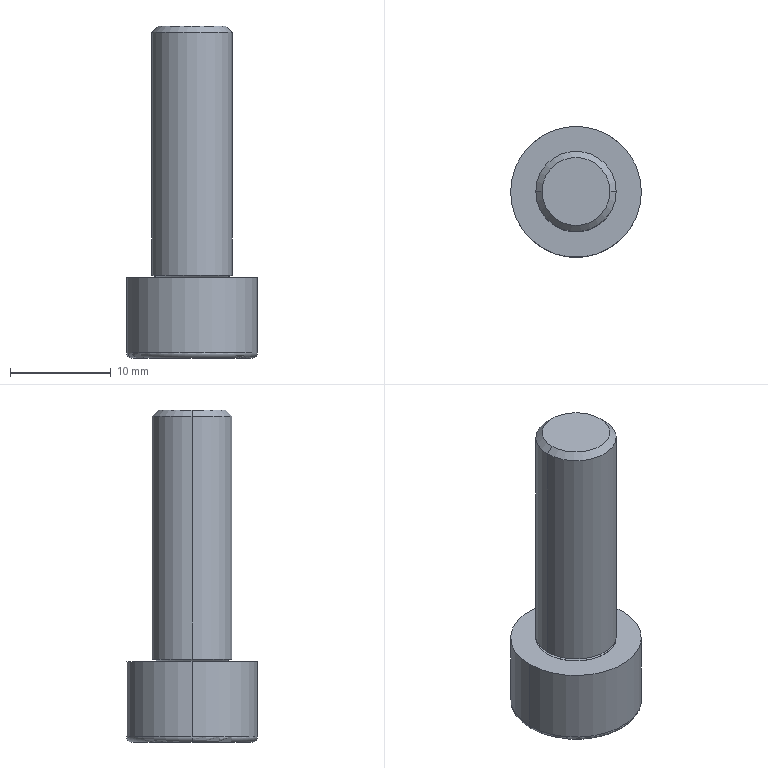Part | SolidWorks | features Attribute 1, Cut 1, Revolution 1 | 1 solid | 27 faces | box 13 x 13 x 33 mm | volume 2217 mm3 | plane 11 | torus 6 | cylinder 6 | cone 4 | commonest cylinder face diameters 8 x4 13 x2
STEP:
#1=CARTESIAN_POINT('',(-3.488,0.,0.01));
#2=VERTEX_POINT('',#1);
#3=CARTESIAN_POINT('',(-3.468,0.,0.03));
#4=VERTEX_POINT('',#3);
#5=CARTESIAN_POINT('',(-3.488,0.,0.03));
#6=DIRECTION('',(0.,-1.,0.));
#7=DIRECTION('',(0.,0.,-1.));
#8=AXIS2_PLACEMENT_3D('',#5,#6,#7);
#9=CIRCLE('',#8,0.02);
#10=EDGE_CURVE('',#2,#4,#9,.T.);
#11=ORIENTED_EDGE('',*,*,#10,.T.);
#12=CARTESIAN_POINT('',(3.468,0.,0.03));
#13=VERTEX_POINT('',#12);
#14=CARTESIAN_POINT('',(0.,0.,0.03));
#15=DIRECTION('',(0.,0.,-1.));
#16=DIRECTION('',(-1.,0.,0.));
#17=AXIS2_PLACEMENT_3D('',#14,#15,#16);
#18=CIRCLE('',#17,3.468);
#19=EDGE_CURVE('',#4,#13,#18,.T.);
#20=ORIENTED_EDGE('',*,*,#19,.T.);
#21=CARTESIAN_POINT('',(3.488,0.,0.01));
#22=VERTEX_POINT('',#21);
#23=CARTESIAN_POINT('',(3.488,0.,0.03));
#24=DIRECTION('',(0.,1.,0.));
#25=DIRECTION('',(-1.,0.,0.));
#26=AXIS2_PLACEMENT_3D('',#23,#24,#25);
#27=CIRCLE('',#26,0.02);
#28=EDGE_CURVE('',#22,#13,#27,.T.);
#29=ORIENTED_EDGE('',*,*,#28,.F.);
#30=CARTESIAN_POINT('',(0.,0.,0.01));
#31=DIRECTION('',(0.,0.,-1.));
#32=DIRECTION('',(-1.,0.,0.));
#33=AXIS2_PLACEMENT_3D('',#30,#31,#32);
#34=CIRCLE('',#33,3.488);
#35=EDGE_CURVE('',#2,#22,#34,.T.);
#36=ORIENTED_EDGE('',*,*,#35,.F.);
#37=EDGE_LOOP('',(#11,#20,#29,#36));
#38=FACE_OUTER_BOUND('',#37,.T.);
#39=CARTESIAN_POINT('',(0.,0.,0.03));
#40=DIRECTION('',(0.,0.,-1.));
#41=DIRECTION('',(-1.,0.,0.));
#42=AXIS2_PLACEMENT_3D('',#39,#40,#41);
#43=TOROIDAL_SURFACE('',#42,3.488,0.02);
#44=ADVANCED_FACE('',(#38),#43,.F.);
#45=ORIENTED_EDGE('',*,*,#28,.T.);
#46=CARTESIAN_POINT('',(0.,0.,0.03));
#47=DIRECTION('',(0.,0.,-1.));
#48=DIRECTION('',(-1.,0.,0.));
#49=AXIS2_PLACEMENT_3D('',#46,#47,#48);
#50=CIRCLE('',#49,3.468);
#51=EDGE_CURVE('',#13,#4,#50,.T.);
#52=ORIENTED_EDGE('',*,*,#51,.T.);
#53=ORIENTED_EDGE('',*,*,#10,.F.);
#54=CARTESIAN_POINT('',(0.,0.,0.01));
#55=DIRECTION('',(0.,0.,-1.));
#56=DIRECTION('',(-1.,0.,0.));
#57=AXIS2_PLACEMENT_3D('',#54,#55,#56);
#58=CIRCLE('',#57,3.488);
#59=EDGE_CURVE('',#22,#2,#58,.T.);
#60=ORIENTED_EDGE('',*,*,#59,.F.);
#61=EDGE_LOOP('',(#45,#52,#53,#60));
#62=FACE_OUTER_BOUND('',#61,.T.);
#63=CARTESIAN_POINT('',(0.,0.,0.03));
#64=DIRECTION('',(0.,0.,-1.));
#65=DIRECTION('',(-1.,0.,0.));
#66=AXIS2_PLACEMENT_3D('',#63,#64,#65);
#67=TOROIDAL_SURFACE('',#66,3.488,0.02);
#68=ADVANCED_FACE('',(#62),#67,.F.);
#69=CARTESIAN_POINT('',(-3.375,0.,25.));
#70=VERTEX_POINT('',#69);
#71=CARTESIAN_POINT('',(3.375,0.,25.));
#72=VERTEX_POINT('',#71);
#73=CARTESIAN_POINT('',(0.,0.,25.));
#74=DIRECTION('',(0.,0.,-1.));
#75=DIRECTION('',(-1.,0.,0.));
#76=AXIS2_PLACEMENT_3D('',#73,#74,#75);
#77=CIRCLE('',#76,3.375);
#78=EDGE_CURVE('',#70,#72,#77,.T.);
#79=ORIENTED_EDGE('',*,*,#78,.T.);
#80=CARTESIAN_POINT('',(4.,0.,24.375));
#81=VERTEX_POINT('',#80);
#82=CARTESIAN_POINT('',(3.375,0.,25.));
#83=DIRECTION('',(0.7071,0.,-0.7071));
#84=VECTOR('',#83,1000.);
#85=LINE('',#82,#84);
#86=EDGE_CURVE('',#72,#81,#85,.T.);
#87=ORIENTED_EDGE('',*,*,#86,.T.);
#88=CARTESIAN_POINT('',(-4.,0.,24.375));
#89=VERTEX_POINT('',#88);
#90=CARTESIAN_POINT('',(0.,0.,24.375));
#91=DIRECTION('',(0.,0.,-1.));
#92=DIRECTION('',(-1.,0.,0.));
#93=AXIS2_PLACEMENT_3D('',#90,#91,#92);
#94=CIRCLE('',#93,4.);
#95=EDGE_CURVE('',#89,#81,#94,.T.);
#96=ORIENTED_EDGE('',*,*,#95,.F.);
#97=CARTESIAN_POINT('',(-3.375,0.,25.));
#98=DIRECTION('',(-0.7071,0.,-0.7071));
#99=VECTOR('',#98,1000.);
#100=LINE('',#97,#99);
#101=EDGE_CURVE('',#70,#89,#100,.T.);
#102=ORIENTED_EDGE('',*,*,#101,.F.);
#103=EDGE_LOOP('',(#79,#87,#96,#102));
#104=FACE_OUTER_BOUND('',#103,.T.);
#105=CARTESIAN_POINT('',(0.,0.,25.));
#106=DIRECTION('',(0.,0.,-1.));
#107=DIRECTION('',(-1.,0.,0.));
#108=AXIS2_PLACEMENT_3D('',#105,#106,#107);
#109=CONICAL_SURFACE('',#108,3.375,0.7854);
#110=ADVANCED_FACE('',(#104),#109,.T.);
#111=ORIENTED_EDGE('',*,*,#95,.T.);
#112=CARTESIAN_POINT('',(4.,0.,0.2375));
#113=VERTEX_POINT('',#112);
#114=CARTESIAN_POINT('',(4.,0.,-10.585));
#115=DIRECTION('',(0.,0.,-1.));
#116=VECTOR('',#115,1000.);
#117=LINE('',#114,#116);
#118=EDGE_CURVE('',#81,#113,#117,.T.);
#119=ORIENTED_EDGE('',*,*,#118,.T.);
#120=CARTESIAN_POINT('',(-4.,0.,0.2375));
#121=VERTEX_POINT('',#120);
#122=CARTESIAN_POINT('',(0.,0.,0.2375));
#123=DIRECTION('',(0.,0.,-1.));
#124=DIRECTION('',(-1.,0.,0.));
#125=AXIS2_PLACEMENT_3D('',#122,#123,#124);
#126=CIRCLE('',#125,4.);
#127=EDGE_CURVE('',#121,#113,#126,.T.);
#128=ORIENTED_EDGE('',*,*,#127,.F.);
#129=CARTESIAN_POINT('',(-4.,0.,-10.585));
#130=DIRECTION('',(0.,0.,-1.));
#131=VECTOR('',#130,1000.);
#132=LINE('',#129,#131);
#133=EDGE_CURVE('',#89,#121,#132,.T.);
#134=ORIENTED_EDGE('',*,*,#133,.F.);
#135=EDGE_LOOP('',(#111,#119,#128,#134));
#136=FACE_OUTER_BOUND('',#135,.T.);
#137=CARTESIAN_POINT('',(0.,0.,-10.585));
#138=DIRECTION('',(0.,0.,-1.));
#139=DIRECTION('',(-1.,0.,0.));
#140=AXIS2_PLACEMENT_3D('',#137,#138,#139);
#141=CYLINDRICAL_SURFACE('',#140,4.);
#142=ADVANCED_FACE('',(#136),#141,.T.);
#143=CARTESIAN_POINT('',(-3.482,0.,0.04879));
#144=VERTEX_POINT('',#143);
#145=CARTESIAN_POINT('',(3.482,0.,0.04879));
#146=VERTEX_POINT('',#145);
#147=CARTESIAN_POINT('',(0.,0.,0.04879));
#148=DIRECTION('',(0.,0.,-1.));
#149=DIRECTION('',(-1.,0.,0.));
#150=AXIS2_PLACEMENT_3D('',#147,#148,#149);
#151=CIRCLE('',#150,3.482);
#152=EDGE_CURVE('',#144,#146,#151,.T.);
#153=ORIENTED_EDGE('',*,*,#152,.F.);
#154=CARTESIAN_POINT('',(-4.,0.,0.2375));
#155=DIRECTION('',(-0.9397,0.,0.342));
#156=VECTOR('',#155,1000.);
#157=LINE('',#154,#156);
#158=EDGE_CURVE('',#144,#121,#157,.T.);
#159=ORIENTED_EDGE('',*,*,#158,.T.);
#160=ORIENTED_EDGE('',*,*,#127,.T.);
#161=CARTESIAN_POINT('',(4.,0.,0.2375));
#162=DIRECTION('',(0.9397,0.,0.342));
#163=VECTOR('',#162,1000.);
#164=LINE('',#161,#163);
#165=EDGE_CURVE('',#146,#113,#164,.T.);
#166=ORIENTED_EDGE('',*,*,#165,.F.);
#167=EDGE_LOOP('',(#153,#159,#160,#166));
#168=FACE_OUTER_BOUND('',#167,.T.);
#169=CARTESIAN_POINT('',(0.,0.,0.2375));
#170=DIRECTION('',(0.,0.,1.));
#171=DIRECTION('',(1.,0.,0.));
#172=AXIS2_PLACEMENT_3D('',#169,#170,#171);
#173=CONICAL_SURFACE('',#172,4.,1.222);
#174=ADVANCED_FACE('',(#168),#173,.T.);
#175=ORIENTED_EDGE('',*,*,#51,.F.);
#176=CARTESIAN_POINT('',(3.488,0.,0.03));
#177=DIRECTION('',(0.,1.,0.));
#178=DIRECTION('',(-1.,0.,0.));
#179=AXIS2_PLACEMENT_3D('',#176,#177,#178);
#180=CIRCLE('',#179,0.02);
#181=EDGE_CURVE('',#13,#146,#180,.T.);
#182=ORIENTED_EDGE('',*,*,#181,.T.);
#183=CARTESIAN_POINT('',(0.,0.,0.04879));
#184=DIRECTION('',(0.,0.,-1.));
#185=DIRECTION('',(-1.,0.,0.));
#186=AXIS2_PLACEMENT_3D('',#183,#184,#185);
#187=CIRCLE('',#186,3.482);
#188=EDGE_CURVE('',#146,#144,#187,.T.);
#189=ORIENTED_EDGE('',*,*,#188,.T.);
#190=CARTESIAN_POINT('',(-3.488,0.,0.03));
#191=DIRECTION('',(0.,-1.,0.));
#192=DIRECTION('',(0.,0.,-1.));
#193=AXIS2_PLACEMENT_3D('',#190,#191,#192);
#194=CIRCLE('',#193,0.02);
#195=EDGE_CURVE('',#4,#144,#194,.T.);
#196=ORIENTED_EDGE('',*,*,#195,.F.);
#197=EDGE_LOOP('',(#175,#182,#189,#196));
#198=FACE_OUTER_BOUND('',#197,.T.);
#199=CARTESIAN_POINT('',(0.,0.,0.03));
#200=DIRECTION('',(0.,0.,-1.));
#201=DIRECTION('',(-1.,0.,0.));
#202=AXIS2_PLACEMENT_3D('',#199,#200,#201);
#203=TOROIDAL_SURFACE('',#202,3.488,0.02);
#204=ADVANCED_FACE('',(#198),#203,.F.);
#205=CARTESIAN_POINT('',(-4.,0.,0.01));
#206=VERTEX_POINT('',#205);
#207=CARTESIAN_POINT('',(4.,0.,0.01));
#208=VERTEX_POINT('',#207);
#209=CARTESIAN_POINT('',(0.,0.,0.01));
#210=DIRECTION('',(0.,0.,-1.));
#211=DIRECTION('',(-1.,0.,0.));
#212=AXIS2_PLACEMENT_3D('',#209,#210,#211);
#213=CIRCLE('',#212,4.);
#214=EDGE_CURVE('',#206,#208,#213,.T.);
#215=ORIENTED_EDGE('',*,*,#214,.T.);
#216=CARTESIAN_POINT('',(4.,0.,0.));
#217=VERTEX_POINT('',#216);
#218=CARTESIAN_POINT('',(4.,0.,-10.585));
#219=DIRECTION('',(0.,0.,-1.));
#220=VECTOR('',#219,1000.);
#221=LINE('',#218,#220);
#222=EDGE_CURVE('',#208,#217,#221,.T.);
#223=ORIENTED_EDGE('',*,*,#222,.T.);
#224=CARTESIAN_POINT('',(-4.,0.,0.));
#225=VERTEX_POINT('',#224);
#226=CARTESIAN_POINT('',(0.,0.,0.));
#227=DIRECTION('',(0.,0.,-1.));
#228=DIRECTION('',(-1.,0.,0.));
#229=AXIS2_PLACEMENT_3D('',#226,#227,#228);
#230=CIRCLE('',#229,4.);
#231=EDGE_CURVE('',#225,#217,#230,.T.);
#232=ORIENTED_EDGE('',*,*,#231,.F.);
#233=CARTESIAN_POINT('',(-4.,0.,-10.585));
#234=DIRECTION('',(0.,0.,-1.));
#235=VECTOR('',#234,1000.);
#236=LINE('',#233,#235);
#237=EDGE_CURVE('',#206,#225,#236,.T.);
#238=ORIENTED_EDGE('',*,*,#237,.F.);
#239=EDGE_LOOP('',(#215,#223,#232,#238));
#240=FACE_OUTER_BOUND('',#239,.T.);
#241=CARTESIAN_POINT('',(0.,0.,-10.585));
#242=DIRECTION('',(0.,0.,-1.));
#243=DIRECTION('',(-1.,0.,0.));
#244=AXIS2_PLACEMENT_3D('',#241,#242,#243);
#245=CYLINDRICAL_SURFACE('',#244,4.);
#246=ADVANCED_FACE('',(#240),#245,.T.);
#247=CARTESIAN_POINT('',(-6.5,0.,0.));
#248=VERTEX_POINT('',#247);
#249=CARTESIAN_POINT('',(6.5,0.,0.));
#250=VERTEX_POINT('',#249);
#251=CARTESIAN_POINT('',(0.,0.,0.));
#252=DIRECTION('',(0.,0.,-1.));
#253=DIRECTION('',(-1.,0.,0.));
#254=AXIS2_PLACEMENT_3D('',#251,#252,#253);
#255=CIRCLE('',#254,6.5);
#256=EDGE_CURVE('',#248,#250,#255,.T.);
#257=ORIENTED_EDGE('',*,*,#256,.T.);
#258=CARTESIAN_POINT('',(6.5,0.,-7.5));
#259=VERTEX_POINT('',#258);
#260=CARTESIAN_POINT('',(6.5,0.,-10.585));
#261=DIRECTION('',(0.,0.,-1.));
#262=VECTOR('',#261,1000.);
#263=LINE('',#260,#262);
#264=EDGE_CURVE('',#250,#259,#263,.T.);
#265=ORIENTED_EDGE('',*,*,#264,.T.);
#266=CARTESIAN_POINT('',(-6.5,0.,-7.5));
#267=VERTEX_POINT('',#266);
#268=CARTESIAN_POINT('',(0.,0.,-7.5));
#269=DIRECTION('',(0.,0.,-1.));
#270=DIRECTION('',(-1.,0.,0.));
#271=AXIS2_PLACEMENT_3D('',#268,#269,#270);
#272=CIRCLE('',#271,6.5);
#273=EDGE_CURVE('',#267,#259,#272,.T.);
#274=ORIENTED_EDGE('',*,*,#273,.F.);
#275=CARTESIAN_POINT('',(-6.5,0.,-10.585));
#276=DIRECTION('',(0.,0.,-1.));
#277=VECTOR('',#276,1000.);
#278=LINE('',#275,#277);
#279=EDGE_CURVE('',#248,#267,#278,.T.);
#280=ORIENTED_EDGE('',*,*,#279,.F.);
#281=EDGE_LOOP('',(#257,#265,#274,#280));
#282=FACE_OUTER_BOUND('',#281,.T.);
#283=CARTESIAN_POINT('',(0.,0.,-10.585));
#284=DIRECTION('',(0.,0.,-1.));
#285=DIRECTION('',(-1.,0.,0.));
#286=AXIS2_PLACEMENT_3D('',#283,#284,#285);
#287=CYLINDRICAL_SURFACE('',#286,6.5);
#288=ADVANCED_FACE('',(#282),#287,.T.);
#289=ORIENTED_EDGE('',*,*,#273,.T.);
#290=CARTESIAN_POINT('',(6.,0.,-8.));
#291=VERTEX_POINT('',#290);
#292=CARTESIAN_POINT('',(6.,0.,-7.5));
#293=DIRECTION('',(0.,1.,0.));
#294=DIRECTION('',(-1.,0.,0.));
#295=AXIS2_PLACEMENT_3D('',#292,#293,#294);
#296=CIRCLE('',#295,0.5);
#297=EDGE_CURVE('',#259,#291,#296,.T.);
#298=ORIENTED_EDGE('',*,*,#297,.T.);
#299=CARTESIAN_POINT('',(-6.,0.,-8.));
#300=VERTEX_POINT('',#299);
#301=CARTESIAN_POINT('',(0.,0.,-8.));
#302=DIRECTION('',(0.,0.,-1.));
#303=DIRECTION('',(-1.,0.,0.));
#304=AXIS2_PLACEMENT_3D('',#301,#302,#303);
#305=CIRCLE('',#304,6.);
#306=EDGE_CURVE('',#300,#291,#305,.T.);
#307=ORIENTED_EDGE('',*,*,#306,.F.);
#308=CARTESIAN_POINT('',(-6.,0.,-7.5));
#309=DIRECTION('',(0.,-1.,0.));
#310=DIRECTION('',(0.,0.,-1.));
#311=AXIS2_PLACEMENT_3D('',#308,#309,#310);
#312=CIRCLE('',#311,0.5);
#313=EDGE_CURVE('',#267,#300,#312,.T.);
#314=ORIENTED_EDGE('',*,*,#313,.F.);
#315=EDGE_LOOP('',(#289,#298,#307,#314));
#316=FACE_OUTER_BOUND('',#315,.T.);
#317=CARTESIAN_POINT('',(0.,0.,-7.5));
#318=DIRECTION('',(0.,0.,-1.));
#319=DIRECTION('',(-1.,0.,0.));
#320=AXIS2_PLACEMENT_3D('',#317,#318,#319);
#321=TOROIDAL_SURFACE('',#320,6.,0.5);
#322=ADVANCED_FACE('',(#316),#321,.T.);
#323=ORIENTED_EDGE('',*,*,#297,.F.);
#324=CARTESIAN_POINT('',(0.,0.,-7.5));
#325=DIRECTION('',(0.,0.,-1.));
#326=DIRECTION('',(-1.,0.,0.));
#327=AXIS2_PLACEMENT_3D('',#324,#325,#326);
#328=CIRCLE('',#327,6.5);
#329=EDGE_CURVE('',#259,#267,#328,.T.);
#330=ORIENTED_EDGE('',*,*,#329,.T.);
#331=ORIENTED_EDGE('',*,*,#313,.T.);
#332=CARTESIAN_POINT('',(0.,0.,-8.));
#333=DIRECTION('',(0.,0.,-1.));
#334=DIRECTION('',(-1.,0.,0.));
#335=AXIS2_PLACEMENT_3D('',#332,#333,#334);
#336=CIRCLE('',#335,6.);
#337=EDGE_CURVE('',#291,#300,#336,.T.);
#338=ORIENTED_EDGE('',*,*,#337,.F.);
#339=EDGE_LOOP('',(#323,#330,#331,#338));
#340=FACE_OUTER_BOUND('',#339,.T.);
#341=CARTESIAN_POINT('',(0.,0.,-7.5));
#342=DIRECTION('',(0.,0.,-1.));
#343=DIRECTION('',(-1.,0.,0.));
#344=AXIS2_PLACEMENT_3D('',#341,#342,#343);
#345=TOROIDAL_SURFACE('',#344,6.,0.5);
#346=ADVANCED_FACE('',(#340),#345,.T.);
#347=ORIENTED_EDGE('',*,*,#264,.F.);
#348=CARTESIAN_POINT('',(0.,0.,0.));
#349=DIRECTION('',(0.,0.,-1.));
#350=DIRECTION('',(-1.,0.,0.));
#351=AXIS2_PLACEMENT_3D('',#348,#349,#350);
#352=CIRCLE('',#351,6.5);
#353=EDGE_CURVE('',#250,#248,#352,.T.);
#354=ORIENTED_EDGE('',*,*,#353,.T.);
#355=ORIENTED_EDGE('',*,*,#279,.T.);
#356=ORIENTED_EDGE('',*,*,#329,.F.);
#357=EDGE_LOOP('',(#347,#354,#355,#356));
#358=FACE_OUTER_BOUND('',#357,.T.);
#359=CARTESIAN_POINT('',(0.,0.,-10.585));
#360=DIRECTION('',(0.,0.,-1.));
#361=DIRECTION('',(-1.,0.,0.));
#362=AXIS2_PLACEMENT_3D('',#359,#360,#361);
#363=CYLINDRICAL_SURFACE('',#362,6.5);
#364=ADVANCED_FACE('',(#358),#363,.T.);
#365=ORIENTED_EDGE('',*,*,#256,.F.);
#366=ORIENTED_EDGE('',*,*,#353,.F.);
#367=EDGE_LOOP('',(#365,#366));
#368=FACE_OUTER_BOUND('',#367,.T.);
#369=ORIENTED_EDGE('',*,*,#231,.T.);
#370=CARTESIAN_POINT('',(0.,0.,0.));
#371=DIRECTION('',(0.,0.,-1.));
#372=DIRECTION('',(-1.,0.,0.));
#373=AXIS2_PLACEMENT_3D('',#370,#371,#372);
#374=CIRCLE('',#373,4.);
#375=EDGE_CURVE('',#217,#225,#374,.T.);
#376=ORIENTED_EDGE('',*,*,#375,.T.);
#377=EDGE_LOOP('',(#369,#376));
#378=FACE_BOUND('',#377,.T.);
#379=CARTESIAN_POINT('',(-6.5,0.,0.));
#380=DIRECTION('',(0.,0.,-1.));
#381=DIRECTION('',(-1.,0.,0.));
#382=AXIS2_PLACEMENT_3D('',#379,#380,#381);
#383=PLANE('',#382);
#384=ADVANCED_FACE('',(#368,#378),#383,.F.);
#385=ORIENTED_EDGE('',*,*,#222,.F.);
#386=CARTESIAN_POINT('',(0.,0.,0.01));
#387=DIRECTION('',(0.,0.,-1.));
#388=DIRECTION('',(-1.,0.,0.));
#389=AXIS2_PLACEMENT_3D('',#386,#387,#388);
#390=CIRCLE('',#389,4.);
#391=EDGE_CURVE('',#208,#206,#390,.T.);
#392=ORIENTED_EDGE('',*,*,#391,.T.);
#393=ORIENTED_EDGE('',*,*,#237,.T.);
#394=ORIENTED_EDGE('',*,*,#375,.F.);
#395=EDGE_LOOP('',(#385,#392,#393,#394));
#396=FACE_OUTER_BOUND('',#395,.T.);
#397=CARTESIAN_POINT('',(0.,0.,-10.585));
#398=DIRECTION('',(0.,0.,-1.));
#399=DIRECTION('',(-1.,0.,0.));
#400=AXIS2_PLACEMENT_3D('',#397,#398,#399);
#401=CYLINDRICAL_SURFACE('',#400,4.);
#402=ADVANCED_FACE('',(#396),#401,.T.);
#403=ORIENTED_EDGE('',*,*,#214,.F.);
#404=ORIENTED_EDGE('',*,*,#391,.F.);
#405=EDGE_LOOP('',(#403,#404));
#406=FACE_OUTER_BOUND('',#405,.T.);
#407=ORIENTED_EDGE('',*,*,#35,.T.);
#408=ORIENTED_EDGE('',*,*,#59,.T.);
#409=EDGE_LOOP('',(#407,#408));
#410=FACE_BOUND('',#409,.T.);
#411=CARTESIAN_POINT('',(-4.,0.,0.01));
#412=DIRECTION('',(0.,0.,-1.));
#413=DIRECTION('',(-1.,0.,0.));
#414=AXIS2_PLACEMENT_3D('',#411,#412,#413);
#415=PLANE('',#414);
#416=ADVANCED_FACE('',(#406,#410),#415,.F.);
#417=ORIENTED_EDGE('',*,*,#19,.F.);
#418=ORIENTED_EDGE('',*,*,#195,.T.);
#419=ORIENTED_EDGE('',*,*,#152,.T.);
#420=ORIENTED_EDGE('',*,*,#181,.F.);
#421=EDGE_LOOP('',(#417,#418,#419,#420));
#422=FACE_OUTER_BOUND('',#421,.T.);
#423=CARTESIAN_POINT('',(0.,0.,0.03));
#424=DIRECTION('',(0.,0.,-1.));
#425=DIRECTION('',(-1.,0.,0.));
#426=AXIS2_PLACEMENT_3D('',#423,#424,#425);
#427=TOROIDAL_SURFACE('',#426,3.488,0.02);
#428=ADVANCED_FACE('',(#422),#427,.F.);
#429=ORIENTED_EDGE('',*,*,#158,.F.);
#430=ORIENTED_EDGE('',*,*,#188,.F.);
#431=ORIENTED_EDGE('',*,*,#165,.T.);
#432=CARTESIAN_POINT('',(0.,0.,0.2375));
#433=DIRECTION('',(0.,0.,-1.));
#434=DIRECTION('',(-1.,0.,0.));
#435=AXIS2_PLACEMENT_3D('',#432,#433,#434);
#436=CIRCLE('',#435,4.);
#437=EDGE_CURVE('',#113,#121,#436,.T.);
#438=ORIENTED_EDGE('',*,*,#437,.T.);
#439=EDGE_LOOP('',(#429,#430,#431,#438));
#440=FACE_OUTER_BOUND('',#439,.T.);
#441=CARTESIAN_POINT('',(0.,0.,0.2375));
#442=DIRECTION('',(0.,0.,1.));
#443=DIRECTION('',(1.,0.,0.));
#444=AXIS2_PLACEMENT_3D('',#441,#442,#443);
#445=CONICAL_SURFACE('',#444,4.,1.222);
#446=ADVANCED_FACE('',(#440),#445,.T.);
#447=ORIENTED_EDGE('',*,*,#118,.F.);
#448=CARTESIAN_POINT('',(0.,0.,24.375));
#449=DIRECTION('',(0.,0.,-1.));
#450=DIRECTION('',(-1.,0.,0.));
#451=AXIS2_PLACEMENT_3D('',#448,#449,#450);
#452=CIRCLE('',#451,4.);
#453=EDGE_CURVE('',#81,#89,#452,.T.);
#454=ORIENTED_EDGE('',*,*,#453,.T.);
#455=ORIENTED_EDGE('',*,*,#133,.T.);
#456=ORIENTED_EDGE('',*,*,#437,.F.);
#457=EDGE_LOOP('',(#447,#454,#455,#456));
#458=FACE_OUTER_BOUND('',#457,.T.);
#459=CARTESIAN_POINT('',(0.,0.,-10.585));
#460=DIRECTION('',(0.,0.,-1.));
#461=DIRECTION('',(-1.,0.,0.));
#462=AXIS2_PLACEMENT_3D('',#459,#460,#461);
#463=CYLINDRICAL_SURFACE('',#462,4.);
#464=ADVANCED_FACE('',(#458),#463,.T.);
#465=ORIENTED_EDGE('',*,*,#86,.F.);
#466=CARTESIAN_POINT('',(0.,0.,25.));
#467=DIRECTION('',(0.,0.,-1.));
#468=DIRECTION('',(-1.,0.,0.));
#469=AXIS2_PLACEMENT_3D('',#466,#467,#468);
#470=CIRCLE('',#469,3.375);
#471=EDGE_CURVE('',#72,#70,#470,.T.);
#472=ORIENTED_EDGE('',*,*,#471,.T.);
#473=ORIENTED_EDGE('',*,*,#101,.T.);
#474=ORIENTED_EDGE('',*,*,#453,.F.);
#475=EDGE_LOOP('',(#465,#472,#473,#474));
#476=FACE_OUTER_BOUND('',#475,.T.);
#477=CARTESIAN_POINT('',(0.,0.,25.));
#478=DIRECTION('',(0.,0.,-1.));
#479=DIRECTION('',(-1.,0.,0.));
#480=AXIS2_PLACEMENT_3D('',#477,#478,#479);
#481=CONICAL_SURFACE('',#480,3.375,0.7854);
#482=ADVANCED_FACE('',(#476),#481,.T.);
#483=ORIENTED_EDGE('',*,*,#78,.F.);
#484=ORIENTED_EDGE('',*,*,#471,.F.);
#485=EDGE_LOOP('',(#483,#484));
#486=FACE_OUTER_BOUND('',#485,.T.);
#487=CARTESIAN_POINT('',(-3.375,0.,25.));
#488=DIRECTION('',(0.,0.,-1.));
#489=DIRECTION('',(-1.,0.,0.));
#490=AXIS2_PLACEMENT_3D('',#487,#488,#489);
#491=PLANE('',#490);
#492=ADVANCED_FACE('',(#486),#491,.F.);
#493=CARTESIAN_POINT('',(3.464,0.,-8.));
#494=VERTEX_POINT('',#493);
#495=CARTESIAN_POINT('',(1.732,-3.,-8.));
#496=VERTEX_POINT('',#495);
#497=CARTESIAN_POINT('',(3.464,0.,-8.));
#498=DIRECTION('',(-0.5,-0.866,0.));
#499=VECTOR('',#498,1000.);
#500=LINE('',#497,#499);
#501=EDGE_CURVE('',#494,#496,#500,.T.);
#502=ORIENTED_EDGE('',*,*,#501,.F.);
#503=CARTESIAN_POINT('',(1.732,3.,-8.));
#504=VERTEX_POINT('',#503);
#505=CARTESIAN_POINT('',(1.732,3.,-8.));
#506=DIRECTION('',(0.5,-0.866,0.));
#507=VECTOR('',#506,1000.);
#508=LINE('',#505,#507);
#509=EDGE_CURVE('',#504,#494,#508,.T.);
#510=ORIENTED_EDGE('',*,*,#509,.F.);
#511=CARTESIAN_POINT('',(-1.732,3.,-8.));
#512=VERTEX_POINT('',#511);
#513=CARTESIAN_POINT('',(-1.732,3.,-8.));
#514=DIRECTION('',(1.,0.,0.));
#515=VECTOR('',#514,1000.);
#516=LINE('',#513,#515);
#517=EDGE_CURVE('',#512,#504,#516,.T.);
#518=ORIENTED_EDGE('',*,*,#517,.F.);
#519=CARTESIAN_POINT('',(-3.464,0.,-8.));
#520=VERTEX_POINT('',#519);
#521=CARTESIAN_POINT('',(-3.464,0.,-8.));
#522=DIRECTION('',(0.5,0.866,0.));
#523=VECTOR('',#522,1000.);
#524=LINE('',#521,#523);
#525=EDGE_CURVE('',#520,#512,#524,.T.);
#526=ORIENTED_EDGE('',*,*,#525,.F.);
#527=CARTESIAN_POINT('',(-1.732,-3.,-8.));
#528=VERTEX_POINT('',#527);
#529=CARTESIAN_POINT('',(-1.732,-3.,-8.));
#530=DIRECTION('',(-0.5,0.866,0.));
#531=VECTOR('',#530,1000.);
#532=LINE('',#529,#531);
#533=EDGE_CURVE('',#528,#520,#532,.T.);
#534=ORIENTED_EDGE('',*,*,#533,.F.);
#535=CARTESIAN_POINT('',(1.732,-3.,-8.));
#536=DIRECTION('',(-1.,0.,0.));
#537=VECTOR('',#536,1000.);
#538=LINE('',#535,#537);
#539=EDGE_CURVE('',#496,#528,#538,.T.);
#540=ORIENTED_EDGE('',*,*,#539,.F.);
#541=EDGE_LOOP('',(#502,#510,#518,#526,#534,#540));
#542=FACE_BOUND('',#541,.T.);
#543=ORIENTED_EDGE('',*,*,#306,.T.);
#544=ORIENTED_EDGE('',*,*,#337,.T.);
#545=EDGE_LOOP('',(#543,#544));
#546=FACE_OUTER_BOUND('',#545,.T.);
#547=CARTESIAN_POINT('',(0.,0.,-8.));
#548=DIRECTION('',(0.,0.,1.));
#549=DIRECTION('',(1.,0.,0.));
#550=AXIS2_PLACEMENT_3D('',#547,#548,#549);
#551=PLANE('',#550);
#552=ADVANCED_FACE('',(#542,#546),#551,.F.);
#553=ORIENTED_EDGE('',*,*,#509,.T.);
#554=CARTESIAN_POINT('',(3.464,0.,-5.));
#555=VERTEX_POINT('',#554);
#556=CARTESIAN_POINT('',(3.464,0.,-5.));
#557=DIRECTION('',(0.,0.,-1.));
#558=VECTOR('',#557,1000.);
#559=LINE('',#556,#558);
#560=EDGE_CURVE('',#555,#494,#559,.T.);
#561=ORIENTED_EDGE('',*,*,#560,.F.);
#562=CARTESIAN_POINT('',(1.732,3.,-5.));
#563=VERTEX_POINT('',#562);
#564=CARTESIAN_POINT('',(1.732,3.,-5.));
#565=DIRECTION('',(0.5,-0.866,0.));
#566=VECTOR('',#565,1000.);
#567=LINE('',#564,#566);
#568=EDGE_CURVE('',#563,#555,#567,.T.);
#569=ORIENTED_EDGE('',*,*,#568,.F.);
#570=CARTESIAN_POINT('',(1.732,3.,-5.));
#571=DIRECTION('',(0.,0.,-1.));
#572=VECTOR('',#571,1000.);
#573=LINE('',#570,#572);
#574=EDGE_CURVE('',#563,#504,#573,.T.);
#575=ORIENTED_EDGE('',*,*,#574,.T.);
#576=EDGE_LOOP('',(#553,#561,#569,#575));
#577=FACE_OUTER_BOUND('',#576,.T.);
#578=CARTESIAN_POINT('',(1.732,3.,-5.));
#579=DIRECTION('',(0.866,0.5,0.));
#580=DIRECTION('',(-0.5,0.866,0.));
#581=AXIS2_PLACEMENT_3D('',#578,#579,#580);
#582=PLANE('',#581);
#583=ADVANCED_FACE('',(#577),#582,.F.);
#584=ORIENTED_EDGE('',*,*,#517,.T.);
#585=ORIENTED_EDGE('',*,*,#574,.F.);
#586=CARTESIAN_POINT('',(-1.732,3.,-5.));
#587=VERTEX_POINT('',#586);
#588=CARTESIAN_POINT('',(-1.732,3.,-5.));
#589=DIRECTION('',(1.,0.,0.));
#590=VECTOR('',#589,1000.);
#591=LINE('',#588,#590);
#592=EDGE_CURVE('',#587,#563,#591,.T.);
#593=ORIENTED_EDGE('',*,*,#592,.F.);
#594=CARTESIAN_POINT('',(-1.732,3.,-5.));
#595=DIRECTION('',(0.,0.,-1.));
#596=VECTOR('',#595,1000.);
#597=LINE('',#594,#596);
#598=EDGE_CURVE('',#587,#512,#597,.T.);
#599=ORIENTED_EDGE('',*,*,#598,.T.);
#600=EDGE_LOOP('',(#584,#585,#593,#599));
#601=FACE_OUTER_BOUND('',#600,.T.);
#602=CARTESIAN_POINT('',(-1.732,3.,-5.));
#603=DIRECTION('',(0.,1.,0.));
#604=DIRECTION('',(-1.,0.,0.));
#605=AXIS2_PLACEMENT_3D('',#602,#603,#604);
#606=PLANE('',#605);
#607=ADVANCED_FACE('',(#601),#606,.F.);
#608=ORIENTED_EDGE('',*,*,#525,.T.);
#609=ORIENTED_EDGE('',*,*,#598,.F.);
#610=CARTESIAN_POINT('',(-3.464,0.,-5.));
#611=VERTEX_POINT('',#610);
#612=CARTESIAN_POINT('',(-3.464,0.,-5.));
#613=DIRECTION('',(0.5,0.866,0.));
#614=VECTOR('',#613,1000.);
#615=LINE('',#612,#614);
#616=EDGE_CURVE('',#611,#587,#615,.T.);
#617=ORIENTED_EDGE('',*,*,#616,.F.);
#618=CARTESIAN_POINT('',(-3.464,0.,-5.));
#619=DIRECTION('',(0.,0.,-1.));
#620=VECTOR('',#619,1000.);
#621=LINE('',#618,#620);
#622=EDGE_CURVE('',#611,#520,#621,.T.);
#623=ORIENTED_EDGE('',*,*,#622,.T.);
#624=EDGE_LOOP('',(#608,#609,#617,#623));
#625=FACE_OUTER_BOUND('',#624,.T.);
#626=CARTESIAN_POINT('',(-3.464,0.,-5.));
#627=DIRECTION('',(-0.866,0.5,0.));
#628=DIRECTION('',(-0.5,-0.866,0.));
#629=AXIS2_PLACEMENT_3D('',#626,#627,#628);
#630=PLANE('',#629);
#631=ADVANCED_FACE('',(#625),#630,.F.);
#632=ORIENTED_EDGE('',*,*,#533,.T.);
#633=ORIENTED_EDGE('',*,*,#622,.F.);
#634=CARTESIAN_POINT('',(-1.732,-3.,-5.));
#635=VERTEX_POINT('',#634);
#636=CARTESIAN_POINT('',(-1.732,-3.,-5.));
#637=DIRECTION('',(-0.5,0.866,0.));
#638=VECTOR('',#637,1000.);
#639=LINE('',#636,#638);
#640=EDGE_CURVE('',#635,#611,#639,.T.);
#641=ORIENTED_EDGE('',*,*,#640,.F.);
#642=CARTESIAN_POINT('',(-1.732,-3.,-5.));
#643=DIRECTION('',(0.,0.,-1.));
#644=VECTOR('',#643,1000.);
#645=LINE('',#642,#644);
#646=EDGE_CURVE('',#635,#528,#645,.T.);
#647=ORIENTED_EDGE('',*,*,#646,.T.);
#648=EDGE_LOOP('',(#632,#633,#641,#647));
#649=FACE_OUTER_BOUND('',#648,.T.);
#650=CARTESIAN_POINT('',(-1.732,-3.,-5.));
#651=DIRECTION('',(-0.866,-0.5,0.));
#652=DIRECTION('',(0.5,-0.866,0.));
#653=AXIS2_PLACEMENT_3D('',#650,#651,#652);
#654=PLANE('',#653);
#655=ADVANCED_FACE('',(#649),#654,.F.);
#656=ORIENTED_EDGE('',*,*,#539,.T.);
#657=ORIENTED_EDGE('',*,*,#646,.F.);
#658=CARTESIAN_POINT('',(1.732,-3.,-5.));
#659=VERTEX_POINT('',#658);
#660=CARTESIAN_POINT('',(1.732,-3.,-5.));
#661=DIRECTION('',(-1.,0.,0.));
#662=VECTOR('',#661,1000.);
#663=LINE('',#660,#662);
#664=EDGE_CURVE('',#659,#635,#663,.T.);
#665=ORIENTED_EDGE('',*,*,#664,.F.);
#666=CARTESIAN_POINT('',(1.732,-3.,-5.));
#667=DIRECTION('',(0.,0.,-1.));
#668=VECTOR('',#667,1000.);
#669=LINE('',#666,#668);
#670=EDGE_CURVE('',#659,#496,#669,.T.);
#671=ORIENTED_EDGE('',*,*,#670,.T.);
#672=EDGE_LOOP('',(#656,#657,#665,#671));
#673=FACE_OUTER_BOUND('',#672,.T.);
#674=CARTESIAN_POINT('',(1.732,-3.,-5.));
#675=DIRECTION('',(0.,-1.,0.));
#676=DIRECTION('',(1.,0.,0.));
#677=AXIS2_PLACEMENT_3D('',#674,#675,#676);
#678=PLANE('',#677);
#679=ADVANCED_FACE('',(#673),#678,.F.);
#680=ORIENTED_EDGE('',*,*,#501,.T.);
#681=ORIENTED_EDGE('',*,*,#670,.F.);
#682=CARTESIAN_POINT('',(3.464,0.,-5.));
#683=DIRECTION('',(-0.5,-0.866,0.));
#684=VECTOR('',#683,1000.);
#685=LINE('',#682,#684);
#686=EDGE_CURVE('',#555,#659,#685,.T.);
#687=ORIENTED_EDGE('',*,*,#686,.F.);
#688=ORIENTED_EDGE('',*,*,#560,.T.);
#689=EDGE_LOOP('',(#680,#681,#687,#688));
#690=FACE_OUTER_BOUND('',#689,.T.);
#691=CARTESIAN_POINT('',(3.464,0.,-5.));
#692=DIRECTION('',(0.866,-0.5,0.));
#693=DIRECTION('',(0.5,0.866,0.));
#694=AXIS2_PLACEMENT_3D('',#691,#692,#693);
#695=PLANE('',#694);
#696=ADVANCED_FACE('',(#690),#695,.F.);
#697=ORIENTED_EDGE('',*,*,#568,.T.);
#698=ORIENTED_EDGE('',*,*,#686,.T.);
#699=ORIENTED_EDGE('',*,*,#664,.T.);
#700=ORIENTED_EDGE('',*,*,#640,.T.);
#701=ORIENTED_EDGE('',*,*,#616,.T.);
#702=ORIENTED_EDGE('',*,*,#592,.T.);
#703=EDGE_LOOP('',(#697,#698,#699,#700,#701,#702));
#704=FACE_OUTER_BOUND('',#703,.T.);
#705=CARTESIAN_POINT('',(1.732,3.,-5.));
#706=DIRECTION('',(0.,0.,1.));
#707=DIRECTION('',(1.,0.,0.));
#708=AXIS2_PLACEMENT_3D('',#705,#706,#707);
#709=PLANE('',#708);
#710=ADVANCED_FACE('',(#704),#709,.F.);
#711=CLOSED_SHELL('',(#44,#68,#110,#142,#174,#204,#246,#288,#322,#346,#364,#384,#402,#416,#428,#446,#464,#482,#492,#552,#583,#607,#631,#655,#679,#696,#710));
#712=MANIFOLD_SOLID_BREP('',#711);
#713=CARTESIAN_POINT('',(0.,0.,0.));
#714=DIRECTION('',(0.,0.,1.));
#715=DIRECTION('',(1.,0.,0.));
#716=AXIS2_PLACEMENT_3D('',#713,#714,#715);
#717=(LENGTH_UNIT()NAMED_UNIT(*)SI_UNIT(.MILLI.,.METRE.));
#718=UNCERTAINTY_MEASURE_WITH_UNIT(LENGTH_MEASURE(0.00001),#717,'','');
#719=(NAMED_UNIT(*)PLANE_ANGLE_UNIT()SI_UNIT($,.RADIAN.));
#720=(NAMED_UNIT(*)SI_UNIT($,.STERADIAN.)SOLID_ANGLE_UNIT());
#721=(GEOMETRIC_REPRESENTATION_CONTEXT(3)GLOBAL_UNCERTAINTY_ASSIGNED_CONTEXT((#718))GLOBAL_UNIT_ASSIGNED_CONTEXT((#717,#719,#720))REPRESENTATION_CONTEXT('',''));
#722=ADVANCED_BREP_SHAPE_REPRESENTATION('',(#712,#716),#721);